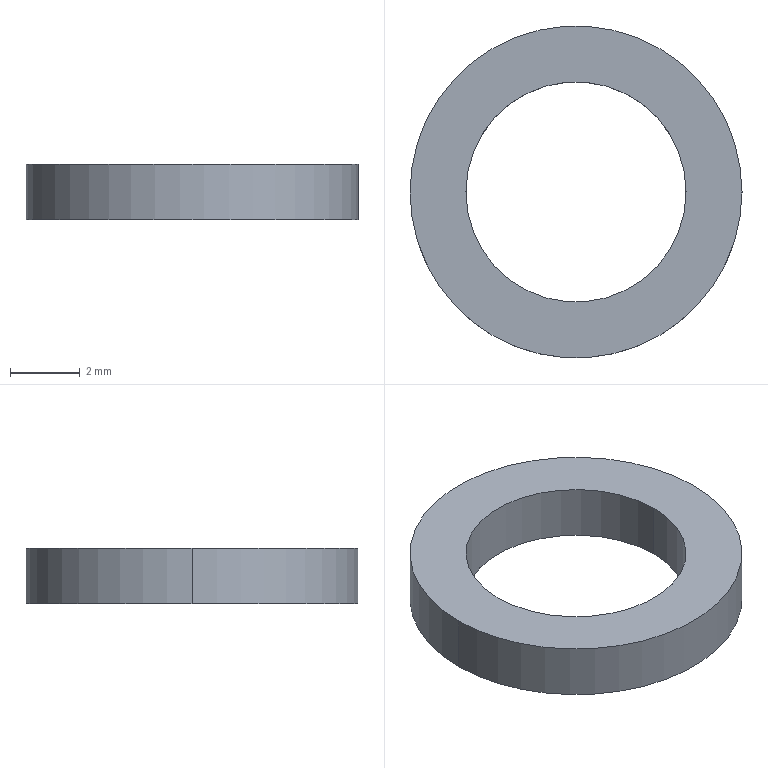Part | STEP file | Washer 2 | 1 solid | 6 faces | box 9.5 x 9.5 x 1.6 mm | volume 63.536 mm3 | cylinder 4 | plane 2 | commonest cylinder face diameters 6.3 x2 9.5 x2
STEP:
#1=CARTESIAN_POINT('',(0.,0.,0.));
#2=DIRECTION('',(0.,0.,1.));
#3=DIRECTION('',(1.,0.,0.));
#4=AXIS2_PLACEMENT_3D('',#1,#2,#3);
#5=CARTESIAN_POINT('',(-3.15,0.,1.6));
#6=VERTEX_POINT('',#5);
#7=CARTESIAN_POINT('',(-3.15,0.,0.));
#8=VERTEX_POINT('',#7);
#9=CARTESIAN_POINT('',(-3.15,0.,1.6));
#10=DIRECTION('',(0.,0.,-1.));
#11=VECTOR('',#10,1.);
#12=LINE('',#9,#11);
#13=CARTESIAN_POINT('',(0.,0.,1.6));
#14=DIRECTION('',(0.,0.,-1.));
#15=DIRECTION('',(-1.,0.,0.));
#16=AXIS2_PLACEMENT_3D('',#13,#14,#15);
#17=CYLINDRICAL_SURFACE('',#16,3.15);
#18=CARTESIAN_POINT('',(6.283,0.));
#19=DIRECTION('',(0.,1.));
#20=VECTOR('',#19,1.);
#21=LINE('',#18,#20);
#22=(GEOMETRIC_REPRESENTATION_CONTEXT(2)PARAMETRIC_REPRESENTATION_CONTEXT()REPRESENTATION_CONTEXT('',''));
#23=DEFINITIONAL_REPRESENTATION('',(#21),#22);
#24=PCURVE('',#17,#23);
#25=CARTESIAN_POINT('',(0.,0.,1.6));
#26=DIRECTION('',(0.,0.,-1.));
#27=DIRECTION('',(-1.,0.,0.));
#28=AXIS2_PLACEMENT_3D('',#25,#26,#27);
#29=CYLINDRICAL_SURFACE('',#28,3.15);
#30=CARTESIAN_POINT('',(0.,0.));
#31=DIRECTION('',(0.,1.));
#32=VECTOR('',#31,1.);
#33=LINE('',#30,#32);
#34=(GEOMETRIC_REPRESENTATION_CONTEXT(2)PARAMETRIC_REPRESENTATION_CONTEXT()REPRESENTATION_CONTEXT('',''));
#35=DEFINITIONAL_REPRESENTATION('',(#33),#34);
#36=PCURVE('',#29,#35);
#37=SURFACE_CURVE('',#12,(#24,#36),.PCURVE_S1.);
#38=EDGE_CURVE('',#6,#8,#37,.T.);
#39=ORIENTED_EDGE('',*,*,#38,.T.);
#40=CARTESIAN_POINT('',(3.15,0.,0.));
#41=VERTEX_POINT('',#40);
#42=CARTESIAN_POINT('',(0.,0.,0.));
#43=DIRECTION('',(0.,0.,1.));
#44=DIRECTION('',(1.,0.,0.));
#45=AXIS2_PLACEMENT_3D('',#42,#43,#44);
#46=CIRCLE('',#45,3.15);
#47=CARTESIAN_POINT('',(9.425,1.6));
#48=DIRECTION('',(-1.,0.));
#49=VECTOR('',#48,1.);
#50=LINE('',#47,#49);
#51=(GEOMETRIC_REPRESENTATION_CONTEXT(2)PARAMETRIC_REPRESENTATION_CONTEXT()REPRESENTATION_CONTEXT('',''));
#52=DEFINITIONAL_REPRESENTATION('',(#50),#51);
#53=PCURVE('',#17,#52);
#54=CARTESIAN_POINT('',(0.,0.,0.));
#55=DIRECTION('',(0.,0.,1.));
#56=DIRECTION('',(1.,0.,0.));
#57=AXIS2_PLACEMENT_3D('',#54,#55,#56);
#58=PLANE('',#57);
#59=CARTESIAN_POINT('',(0.,0.));
#60=DIRECTION('',(1.,0.));
#61=AXIS2_PLACEMENT_2D('',#59,#60);
#62=CIRCLE('',#61,3.15);
#63=(GEOMETRIC_REPRESENTATION_CONTEXT(2)PARAMETRIC_REPRESENTATION_CONTEXT()REPRESENTATION_CONTEXT('',''));
#64=DEFINITIONAL_REPRESENTATION('',(#62),#63);
#65=PCURVE('',#58,#64);
#66=SURFACE_CURVE('',#46,(#53,#65),.PCURVE_S1.);
#67=EDGE_CURVE('',#8,#41,#66,.T.);
#68=ORIENTED_EDGE('',*,*,#67,.T.);
#69=CARTESIAN_POINT('',(3.15,0.,1.6));
#70=VERTEX_POINT('',#69);
#71=CARTESIAN_POINT('',(3.15,0.,1.6));
#72=DIRECTION('',(0.,0.,-1.));
#73=VECTOR('',#72,1.);
#74=LINE('',#71,#73);
#75=CARTESIAN_POINT('',(3.142,0.));
#76=DIRECTION('',(0.,1.));
#77=VECTOR('',#76,1.);
#78=LINE('',#75,#77);
#79=(GEOMETRIC_REPRESENTATION_CONTEXT(2)PARAMETRIC_REPRESENTATION_CONTEXT()REPRESENTATION_CONTEXT('',''));
#80=DEFINITIONAL_REPRESENTATION('',(#78),#79);
#81=PCURVE('',#17,#80);
#82=CARTESIAN_POINT('',(3.142,0.));
#83=DIRECTION('',(0.,1.));
#84=VECTOR('',#83,1.);
#85=LINE('',#82,#84);
#86=(GEOMETRIC_REPRESENTATION_CONTEXT(2)PARAMETRIC_REPRESENTATION_CONTEXT()REPRESENTATION_CONTEXT('',''));
#87=DEFINITIONAL_REPRESENTATION('',(#85),#86);
#88=PCURVE('',#29,#87);
#89=SURFACE_CURVE('',#74,(#81,#88),.PCURVE_S1.);
#90=EDGE_CURVE('',#70,#41,#89,.T.);
#91=ORIENTED_EDGE('',*,*,#90,.F.);
#92=CARTESIAN_POINT('',(0.,0.,1.6));
#93=DIRECTION('',(0.,0.,1.));
#94=DIRECTION('',(1.,0.,0.));
#95=AXIS2_PLACEMENT_3D('',#92,#93,#94);
#96=CIRCLE('',#95,3.15);
#97=CARTESIAN_POINT('',(9.425,0.));
#98=DIRECTION('',(-1.,0.));
#99=VECTOR('',#98,1.);
#100=LINE('',#97,#99);
#101=(GEOMETRIC_REPRESENTATION_CONTEXT(2)PARAMETRIC_REPRESENTATION_CONTEXT()REPRESENTATION_CONTEXT('',''));
#102=DEFINITIONAL_REPRESENTATION('',(#100),#101);
#103=PCURVE('',#17,#102);
#104=CARTESIAN_POINT('',(0.,0.,1.6));
#105=DIRECTION('',(0.,0.,1.));
#106=DIRECTION('',(1.,0.,0.));
#107=AXIS2_PLACEMENT_3D('',#104,#105,#106);
#108=PLANE('',#107);
#109=CARTESIAN_POINT('',(0.,0.));
#110=DIRECTION('',(1.,0.));
#111=AXIS2_PLACEMENT_2D('',#109,#110);
#112=CIRCLE('',#111,3.15);
#113=(GEOMETRIC_REPRESENTATION_CONTEXT(2)PARAMETRIC_REPRESENTATION_CONTEXT()REPRESENTATION_CONTEXT('',''));
#114=DEFINITIONAL_REPRESENTATION('',(#112),#113);
#115=PCURVE('',#108,#114);
#116=SURFACE_CURVE('',#96,(#103,#115),.PCURVE_S1.);
#117=EDGE_CURVE('',#6,#70,#116,.T.);
#118=ORIENTED_EDGE('',*,*,#117,.F.);
#119=EDGE_LOOP('',(#39,#68,#91,#118));
#120=FACE_BOUND('',#119,.F.);
#121=ADVANCED_FACE('',(#120),#17,.F.);
#122=CARTESIAN_POINT('',(4.75,0.,1.6));
#123=VERTEX_POINT('',#122);
#124=CARTESIAN_POINT('',(-4.75,0.,1.6));
#125=VERTEX_POINT('',#124);
#126=CARTESIAN_POINT('',(0.,0.,1.6));
#127=DIRECTION('',(0.,0.,1.));
#128=DIRECTION('',(1.,0.,0.));
#129=AXIS2_PLACEMENT_3D('',#126,#127,#128);
#130=CIRCLE('',#129,4.75);
#131=CARTESIAN_POINT('',(0.,0.,1.6));
#132=DIRECTION('',(0.,0.,-1.));
#133=DIRECTION('',(-1.,0.,0.));
#134=AXIS2_PLACEMENT_3D('',#131,#132,#133);
#135=CYLINDRICAL_SURFACE('',#134,4.75);
#136=CARTESIAN_POINT('',(3.142,0.));
#137=DIRECTION('',(-1.,0.));
#138=VECTOR('',#137,1.);
#139=LINE('',#136,#138);
#140=(GEOMETRIC_REPRESENTATION_CONTEXT(2)PARAMETRIC_REPRESENTATION_CONTEXT()REPRESENTATION_CONTEXT('',''));
#141=DEFINITIONAL_REPRESENTATION('',(#139),#140);
#142=PCURVE('',#135,#141);
#143=CARTESIAN_POINT('',(0.,0.));
#144=DIRECTION('',(1.,0.));
#145=AXIS2_PLACEMENT_2D('',#143,#144);
#146=CIRCLE('',#145,4.75);
#147=(GEOMETRIC_REPRESENTATION_CONTEXT(2)PARAMETRIC_REPRESENTATION_CONTEXT()REPRESENTATION_CONTEXT('',''));
#148=DEFINITIONAL_REPRESENTATION('',(#146),#147);
#149=PCURVE('',#108,#148);
#150=SURFACE_CURVE('',#130,(#142,#149),.PCURVE_S1.);
#151=EDGE_CURVE('',#123,#125,#150,.T.);
#152=ORIENTED_EDGE('',*,*,#151,.F.);
#153=CARTESIAN_POINT('',(4.75,0.,0.));
#154=VERTEX_POINT('',#153);
#155=CARTESIAN_POINT('',(4.75,0.,1.6));
#156=DIRECTION('',(0.,0.,-1.));
#157=VECTOR('',#156,1.);
#158=LINE('',#155,#157);
#159=CARTESIAN_POINT('',(3.142,0.));
#160=DIRECTION('',(0.,1.));
#161=VECTOR('',#160,1.);
#162=LINE('',#159,#161);
#163=(GEOMETRIC_REPRESENTATION_CONTEXT(2)PARAMETRIC_REPRESENTATION_CONTEXT()REPRESENTATION_CONTEXT('',''));
#164=DEFINITIONAL_REPRESENTATION('',(#162),#163);
#165=PCURVE('',#135,#164);
#166=CARTESIAN_POINT('',(0.,0.,1.6));
#167=DIRECTION('',(0.,0.,-1.));
#168=DIRECTION('',(-1.,0.,0.));
#169=AXIS2_PLACEMENT_3D('',#166,#167,#168);
#170=CYLINDRICAL_SURFACE('',#169,4.75);
#171=CARTESIAN_POINT('',(3.142,0.));
#172=DIRECTION('',(0.,1.));
#173=VECTOR('',#172,1.);
#174=LINE('',#171,#173);
#175=(GEOMETRIC_REPRESENTATION_CONTEXT(2)PARAMETRIC_REPRESENTATION_CONTEXT()REPRESENTATION_CONTEXT('',''));
#176=DEFINITIONAL_REPRESENTATION('',(#174),#175);
#177=PCURVE('',#170,#176);
#178=SURFACE_CURVE('',#158,(#165,#177),.PCURVE_S1.);
#179=EDGE_CURVE('',#123,#154,#178,.T.);
#180=ORIENTED_EDGE('',*,*,#179,.T.);
#181=CARTESIAN_POINT('',(-4.75,0.,0.));
#182=VERTEX_POINT('',#181);
#183=CARTESIAN_POINT('',(0.,0.,0.));
#184=DIRECTION('',(0.,0.,1.));
#185=DIRECTION('',(1.,0.,0.));
#186=AXIS2_PLACEMENT_3D('',#183,#184,#185);
#187=CIRCLE('',#186,4.75);
#188=CARTESIAN_POINT('',(3.142,1.6));
#189=DIRECTION('',(-1.,0.));
#190=VECTOR('',#189,1.);
#191=LINE('',#188,#190);
#192=(GEOMETRIC_REPRESENTATION_CONTEXT(2)PARAMETRIC_REPRESENTATION_CONTEXT()REPRESENTATION_CONTEXT('',''));
#193=DEFINITIONAL_REPRESENTATION('',(#191),#192);
#194=PCURVE('',#135,#193);
#195=CARTESIAN_POINT('',(0.,0.));
#196=DIRECTION('',(1.,0.));
#197=AXIS2_PLACEMENT_2D('',#195,#196);
#198=CIRCLE('',#197,4.75);
#199=(GEOMETRIC_REPRESENTATION_CONTEXT(2)PARAMETRIC_REPRESENTATION_CONTEXT()REPRESENTATION_CONTEXT('',''));
#200=DEFINITIONAL_REPRESENTATION('',(#198),#199);
#201=PCURVE('',#58,#200);
#202=SURFACE_CURVE('',#187,(#194,#201),.PCURVE_S1.);
#203=EDGE_CURVE('',#154,#182,#202,.T.);
#204=ORIENTED_EDGE('',*,*,#203,.T.);
#205=CARTESIAN_POINT('',(-4.75,0.,1.6));
#206=DIRECTION('',(0.,0.,-1.));
#207=VECTOR('',#206,1.);
#208=LINE('',#205,#207);
#209=CARTESIAN_POINT('',(0.,0.));
#210=DIRECTION('',(0.,1.));
#211=VECTOR('',#210,1.);
#212=LINE('',#209,#211);
#213=(GEOMETRIC_REPRESENTATION_CONTEXT(2)PARAMETRIC_REPRESENTATION_CONTEXT()REPRESENTATION_CONTEXT('',''));
#214=DEFINITIONAL_REPRESENTATION('',(#212),#213);
#215=PCURVE('',#135,#214);
#216=CARTESIAN_POINT('',(6.283,0.));
#217=DIRECTION('',(0.,1.));
#218=VECTOR('',#217,1.);
#219=LINE('',#216,#218);
#220=(GEOMETRIC_REPRESENTATION_CONTEXT(2)PARAMETRIC_REPRESENTATION_CONTEXT()REPRESENTATION_CONTEXT('',''));
#221=DEFINITIONAL_REPRESENTATION('',(#219),#220);
#222=PCURVE('',#170,#221);
#223=SURFACE_CURVE('',#208,(#215,#222),.PCURVE_S1.);
#224=EDGE_CURVE('',#125,#182,#223,.T.);
#225=ORIENTED_EDGE('',*,*,#224,.F.);
#226=EDGE_LOOP('',(#152,#180,#204,#225));
#227=FACE_BOUND('',#226,.T.);
#228=ADVANCED_FACE('',(#227),#135,.T.);
#229=CARTESIAN_POINT('',(0.,0.,1.6));
#230=DIRECTION('',(0.,0.,1.));
#231=DIRECTION('',(1.,0.,0.));
#232=AXIS2_PLACEMENT_3D('',#229,#230,#231);
#233=CIRCLE('',#232,4.75);
#234=CARTESIAN_POINT('',(0.,0.));
#235=DIRECTION('',(1.,0.));
#236=AXIS2_PLACEMENT_2D('',#234,#235);
#237=CIRCLE('',#236,4.75);
#238=(GEOMETRIC_REPRESENTATION_CONTEXT(2)PARAMETRIC_REPRESENTATION_CONTEXT()REPRESENTATION_CONTEXT('',''));
#239=DEFINITIONAL_REPRESENTATION('',(#237),#238);
#240=PCURVE('',#108,#239);
#241=CARTESIAN_POINT('',(9.425,0.));
#242=DIRECTION('',(-1.,0.));
#243=VECTOR('',#242,1.);
#244=LINE('',#241,#243);
#245=(GEOMETRIC_REPRESENTATION_CONTEXT(2)PARAMETRIC_REPRESENTATION_CONTEXT()REPRESENTATION_CONTEXT('',''));
#246=DEFINITIONAL_REPRESENTATION('',(#244),#245);
#247=PCURVE('',#170,#246);
#248=SURFACE_CURVE('',#233,(#240,#247),.PCURVE_S1.);
#249=EDGE_CURVE('',#125,#123,#248,.T.);
#250=ORIENTED_EDGE('',*,*,#249,.T.);
#251=ORIENTED_EDGE('',*,*,#151,.T.);
#252=EDGE_LOOP('',(#250,#251));
#253=FACE_BOUND('',#252,.T.);
#254=ORIENTED_EDGE('',*,*,#117,.F.);
#255=CARTESIAN_POINT('',(0.,0.,1.6));
#256=DIRECTION('',(0.,0.,1.));
#257=DIRECTION('',(1.,0.,0.));
#258=AXIS2_PLACEMENT_3D('',#255,#256,#257);
#259=CIRCLE('',#258,3.15);
#260=CARTESIAN_POINT('',(0.,0.));
#261=DIRECTION('',(1.,0.));
#262=AXIS2_PLACEMENT_2D('',#260,#261);
#263=CIRCLE('',#262,3.15);
#264=(GEOMETRIC_REPRESENTATION_CONTEXT(2)PARAMETRIC_REPRESENTATION_CONTEXT()REPRESENTATION_CONTEXT('',''));
#265=DEFINITIONAL_REPRESENTATION('',(#263),#264);
#266=PCURVE('',#108,#265);
#267=CARTESIAN_POINT('',(3.142,0.));
#268=DIRECTION('',(-1.,0.));
#269=VECTOR('',#268,1.);
#270=LINE('',#267,#269);
#271=(GEOMETRIC_REPRESENTATION_CONTEXT(2)PARAMETRIC_REPRESENTATION_CONTEXT()REPRESENTATION_CONTEXT('',''));
#272=DEFINITIONAL_REPRESENTATION('',(#270),#271);
#273=PCURVE('',#29,#272);
#274=SURFACE_CURVE('',#259,(#266,#273),.PCURVE_S1.);
#275=EDGE_CURVE('',#70,#6,#274,.T.);
#276=ORIENTED_EDGE('',*,*,#275,.F.);
#277=EDGE_LOOP('',(#254,#276));
#278=FACE_BOUND('',#277,.T.);
#279=ADVANCED_FACE('',(#253,#278),#108,.T.);
#280=CARTESIAN_POINT('',(0.,0.,0.));
#281=DIRECTION('',(0.,0.,1.));
#282=DIRECTION('',(1.,0.,0.));
#283=AXIS2_PLACEMENT_3D('',#280,#281,#282);
#284=CIRCLE('',#283,4.75);
#285=CARTESIAN_POINT('',(0.,0.));
#286=DIRECTION('',(1.,0.));
#287=AXIS2_PLACEMENT_2D('',#285,#286);
#288=CIRCLE('',#287,4.75);
#289=(GEOMETRIC_REPRESENTATION_CONTEXT(2)PARAMETRIC_REPRESENTATION_CONTEXT()REPRESENTATION_CONTEXT('',''));
#290=DEFINITIONAL_REPRESENTATION('',(#288),#289);
#291=PCURVE('',#58,#290);
#292=CARTESIAN_POINT('',(9.425,1.6));
#293=DIRECTION('',(-1.,0.));
#294=VECTOR('',#293,1.);
#295=LINE('',#292,#294);
#296=(GEOMETRIC_REPRESENTATION_CONTEXT(2)PARAMETRIC_REPRESENTATION_CONTEXT()REPRESENTATION_CONTEXT('',''));
#297=DEFINITIONAL_REPRESENTATION('',(#295),#296);
#298=PCURVE('',#170,#297);
#299=SURFACE_CURVE('',#284,(#291,#298),.PCURVE_S1.);
#300=EDGE_CURVE('',#182,#154,#299,.T.);
#301=ORIENTED_EDGE('',*,*,#300,.F.);
#302=ORIENTED_EDGE('',*,*,#203,.F.);
#303=EDGE_LOOP('',(#301,#302));
#304=FACE_BOUND('',#303,.T.);
#305=ORIENTED_EDGE('',*,*,#67,.T.);
#306=CARTESIAN_POINT('',(0.,0.,0.));
#307=DIRECTION('',(0.,0.,1.));
#308=DIRECTION('',(1.,0.,0.));
#309=AXIS2_PLACEMENT_3D('',#306,#307,#308);
#310=CIRCLE('',#309,3.15);
#311=CARTESIAN_POINT('',(0.,0.));
#312=DIRECTION('',(1.,0.));
#313=AXIS2_PLACEMENT_2D('',#311,#312);
#314=CIRCLE('',#313,3.15);
#315=(GEOMETRIC_REPRESENTATION_CONTEXT(2)PARAMETRIC_REPRESENTATION_CONTEXT()REPRESENTATION_CONTEXT('',''));
#316=DEFINITIONAL_REPRESENTATION('',(#314),#315);
#317=PCURVE('',#58,#316);
#318=CARTESIAN_POINT('',(3.142,1.6));
#319=DIRECTION('',(-1.,0.));
#320=VECTOR('',#319,1.);
#321=LINE('',#318,#320);
#322=(GEOMETRIC_REPRESENTATION_CONTEXT(2)PARAMETRIC_REPRESENTATION_CONTEXT()REPRESENTATION_CONTEXT('',''));
#323=DEFINITIONAL_REPRESENTATION('',(#321),#322);
#324=PCURVE('',#29,#323);
#325=SURFACE_CURVE('',#310,(#317,#324),.PCURVE_S1.);
#326=EDGE_CURVE('',#41,#8,#325,.T.);
#327=ORIENTED_EDGE('',*,*,#326,.T.);
#328=EDGE_LOOP('',(#305,#327));
#329=FACE_BOUND('',#328,.T.);
#330=ADVANCED_FACE('',(#304,#329),#58,.F.);
#331=ORIENTED_EDGE('',*,*,#179,.F.);
#332=ORIENTED_EDGE('',*,*,#249,.F.);
#333=ORIENTED_EDGE('',*,*,#224,.T.);
#334=ORIENTED_EDGE('',*,*,#300,.T.);
#335=EDGE_LOOP('',(#331,#332,#333,#334));
#336=FACE_BOUND('',#335,.T.);
#337=ADVANCED_FACE('',(#336),#170,.T.);
#338=ORIENTED_EDGE('',*,*,#326,.T.);
#339=ORIENTED_EDGE('',*,*,#38,.F.);
#340=ORIENTED_EDGE('',*,*,#275,.F.);
#341=ORIENTED_EDGE('',*,*,#90,.T.);
#342=EDGE_LOOP('',(#338,#339,#340,#341));
#343=FACE_BOUND('',#342,.F.);
#344=ADVANCED_FACE('',(#343),#29,.F.);
#345=CLOSED_SHELL('',(#121,#228,#279,#330,#337,#344));
#346=MANIFOLD_SOLID_BREP('',#345);
#347=(LENGTH_UNIT()NAMED_UNIT(*)SI_UNIT(.MILLI.,.METRE.));
#348=UNCERTAINTY_MEASURE_WITH_UNIT(LENGTH_MEASURE(0.0000001),#347,'','');
#349=(NAMED_UNIT(*)PLANE_ANGLE_UNIT()SI_UNIT($,.RADIAN.));
#350=(NAMED_UNIT(*)SI_UNIT($,.STERADIAN.)SOLID_ANGLE_UNIT());
#351=(GEOMETRIC_REPRESENTATION_CONTEXT(3)GLOBAL_UNCERTAINTY_ASSIGNED_CONTEXT((#348))GLOBAL_UNIT_ASSIGNED_CONTEXT((#347,#349,#350))REPRESENTATION_CONTEXT('',''));
#352=ADVANCED_BREP_SHAPE_REPRESENTATION('',(#4,#346),#351);